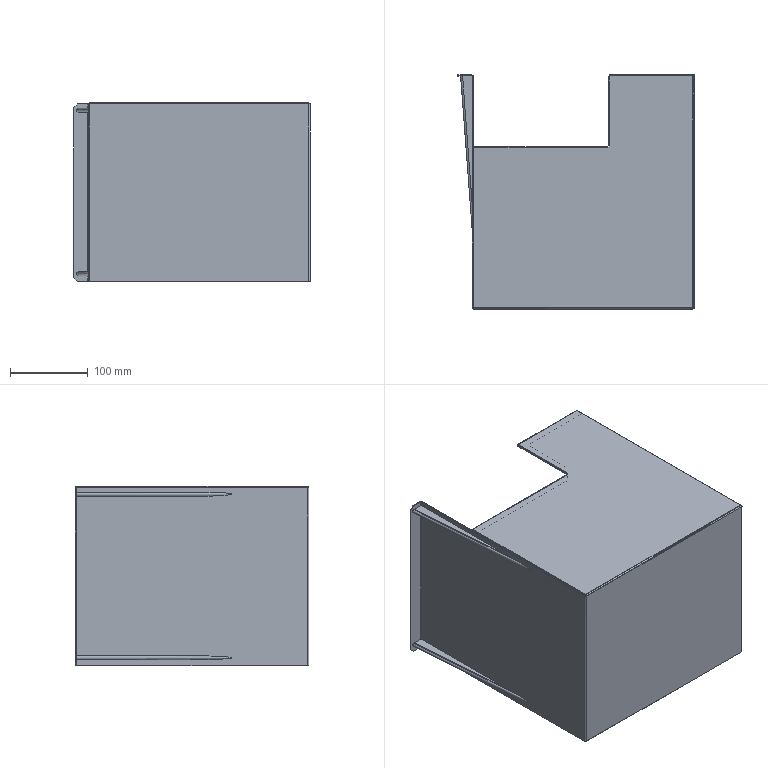Part | STEP file | Guide wheel mechanism revised.sldasm-Part-331 | 1 solid | 83 faces | box 303.8 x 300 x 230 mm | volume 338755 mm3 | plane 53 | cylinder 22 | spline 8 | commonest cylinder face diameters 1.473 x6 3.873 x6 0.1 x3 2.5 x3 2.6 x2 5 x2